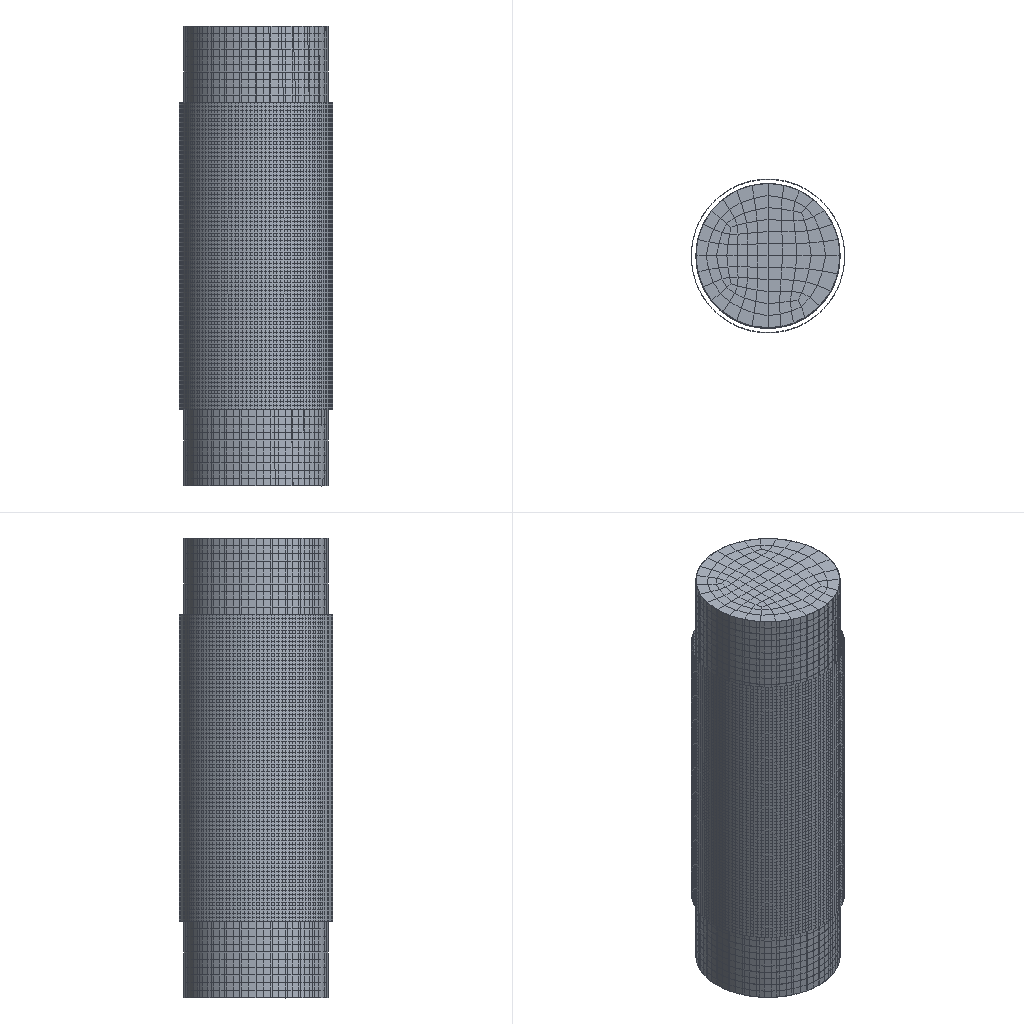Simulation study | abaqus
Set-up summary:
category,name,step,type,value,unit,region
solver,abaqus
solver,version,,,Abaqus/Standard 2020
units,not stated in the deck,,not stated
analysis,deck,,static,static
load_step,Step-1,Step-1,static,nlgeom=True
contact,interactions,,,general=1 pairs=0 ties=1
load_step,requested,,,1
mesh,nodes,,,19323
mesh,elements,,,18438
element_type,S4,,shell,14280
element_type,C3D8,,solid,3540
element_type,R3D3,,rigid,8
element_type,R3D4,,rigid,610
load,load commands in deck,,count,1
bc,support commands in deck,,count,7
material,CONCRETE,,in results
material,PLATE,,in results
material,STEEL,,in results
material,T300/M18,,in results
check,setup vs results,,match,"per instance, exact: element labels, types and connectivity; labels of the nodes the elements use; coordinates of those nodes at SINGLE_PRECISION in 2 of 5 instance(s)"
Abaqus input file, long lists of numbers shortened:
*Heading
** Job name: Job-2 Model name: 3-F1-D-Copy
** Generated by: Abaqus/CAE 2020
*Preprint, echo=NO, model=NO, history=NO, contact=NO
**
** PARTS
**
*Part, name=CFRP
*Node
      1,          50.,           0.,          75.
      2,          50.,           0.,         125.
** (10204 more lines like these left out)
*Element, type=S4
    1,     1,     5,   505,   630
    2,     5,     6,   506,   505
** (10078 more lines like these left out)
*Elset, elset=COMPOSITELAYUP-1-1, generate
     1,  10080,      1
** Region: (COMPOSITELAYUP-1-1: Generated From Layup)
*Elset, elset=COMPOSITELAYUP-1-1-1, generate
     1,  10080,      1
** Section: COMPOSITELAYUP-1-1
*Shell Section, elset=COMPOSITELAYUP-1-1-1, composite, offset=SNEG, layup=COMPOSITELAYUP-1
0.3, 5, T300/M18, 0., 层-1
*End Part
**
*Part, name=con
*Node
      1,           0.,           0.,         300.
      2,           0.,         -47.,         300.
** (4121 more lines like these left out)
*Element, type=C3D8
  1,  407,  408, 1902, 1729,   14,   15,  245,  244
  2,  408,  409, 1903, 1902,   15,   16,  246,  245
** (3538 more lines like these left out)
*Nset, nset=Set-8, generate
    1,  4123,     1
*Elset, elset=Set-8, generate
    1,  3540,     1
** Section: Section-1-_PICKEDSET2
*Solid Section, elset=Set-8, material=CONCRETE
,
*End Part
**
*Part, name="perforated steel"
*Node
      1,  -40.703,        -23.5,         125.
      2,  -30.256,  -35.967,    141.256
** (4372 more lines like these left out)
*Element, type=S4
   1,    1,   63,  919,   82
   2,   63,   64,  920,  919
** (4198 more lines like these left out)
*Nset, nset=_PICKEDSET2_#2, internal, generate
    1,  4374,     1
*Elset, elset=_PICKEDSET2_#2, internal, generate
    1,  4200,     1
*Nset, nset="Edge Seeds-3"
   2,   3,   4,   7,  10,  11,  13,  15,  17,  18,  20,  22,  24,  25,  27,  28
  30,  32,  33,  35,  36,  38,  40,  41,  43,  44,  45,  46,  47,  48,  67,  68
** (13 more lines like these left out)
*Elset, elset="Edge Seeds-3"
    5,   10,   15,   20,   25,   30,   35,   40,   45,   50,   51,   56,   61,   66,   71,   76
   81,   86,   91,   96,  101,  106,  111,  116,  121,  126,  131,  136,  141,  146,  151,  156
** (13 more lines like these left out)
** Section: Section-2-_PICKEDSET2_#2
*Shell Section, elset=_PICKEDSET2_#2, material=STEEL, offset=SNEG
3., 9
*End Part
**
*Part, name=rigid
*Node
      1,   48.014,  -57.617,          40.
      2,   48.014,  -57.617,           0.
** (307 more lines like these left out)
*Element, type=R3D4
 1,   1,   3,  63,  93
 2,   3,   4,  64,  63
** (303 more lines like these left out)
*Element, type=R3D3
94, 182, 212, 165
95, 192, 191, 181
** (2 more lines like these left out)
*Node
    310,           0., -4.59242545e-15,          40.
*Nset, nset=rigid-RefPt_, internal
310,
*Elset, elset=rigid, generate
   1,  309,    1
*End Part
**
**
** ASSEMBLY
**
*Assembly, name=Assembly
**
*Instance, name="perforated steel-1", part="perforated steel"
*End Instance
**
*Instance, name=CFRP-1, part=CFRP
          0.,           0.,          50.
*End Instance
**
*Instance, name=con-1, part=con
*End Instance
**
*Instance, name=rigid-1, part=rigid
          0.,           0.,         -40.
*End Instance
**
*Instance, name=rigid-2, part=rigid
          0.,           0.,         300.
*End Instance
**
*Nset, nset=Set-35, instance=rigid-2
 310,
*Nset, nset=Set-36, instance=rigid-1
 310,
*Elset, elset=__PICKEDSURF62_E3, internal, instance="perforated steel-1"
 2291, 2292, 2293, 2294, 2295, 2296, 2297, 2298, 2299, 2300, 2791, 2792, 2793, 2794, 2795, 2796
 2797, 2798, 2799, 2800, 3291, 3292, 3293, 3294, 3295, 3296, 3297, 3298, 3299, 3300, 3591, 3592
** (2 more lines like these left out)
*Elset, elset=__PICKEDSURF63_E3, internal, instance="perforated steel-1"
 1141, 1142, 1143, 1144, 1145, 1146, 1147, 1148, 1149, 1150, 1441, 1442, 1443, 1444, 1445, 1446
 1447, 1448, 1449, 1450, 1741, 1742, 1743, 1744, 1745, 1746, 1747, 1748, 1749, 1750, 2041, 2042
** (2 more lines like these left out)
*Elset, elset=__PICKEDSURF64_SNEG, internal, instance="perforated steel-1", generate
    1,  4200,     1
*Elset, elset=__PICKEDSURF71_SPOS, internal, instance="perforated steel-1"
    1,    2,    3,    4,    5,    6,    7,    8,    9,   10,   11,   12,   13,   14,   15,   16
   17,   18,   19,   20,   21,   22,   23,   24,   25,   26,   27,   28,   29,   30,   31,   32
** (73 more lines like these left out)
*Elset, elset=__PICKEDSURF72_SPOS, internal, instance="perforated steel-1"
  901,  902,  903,  904,  905,  906,  907,  908,  909,  910,  911,  912,  913,  914,  915,  916
  917,  918,  919,  920,  921,  922,  923,  924,  925,  926,  927,  928,  929,  930,  931,  932
** (92 more lines like these left out)
*Elset, elset=__PICKEDSURF73_SNEG, internal, instance=CFRP-1, generate
  6301,  10080,      1
*Elset, elset=__PICKEDSURF74_SNEG, internal, instance=CFRP-1, generate
    1,  2520,     1
*Elset, elset=__PICKEDSURF75_SPOS, internal, instance="perforated steel-1"
 2051, 2052, 2053, 2054, 2055, 2056, 2057, 2058, 2059, 2060, 2061, 2062, 2063, 2064, 2065, 2066
 2067, 2068, 2069, 2070, 2071, 2072, 2073, 2074, 2075, 2076, 2077, 2078, 2079, 2080, 2081, 2082
** (92 more lines like these left out)
*Elset, elset=__PICKEDSURF76_SNEG, internal, instance=CFRP-1, generate
 2521,  6300,     1
*Elset, elset=_m_Surf-6_E3, internal, instance="perforated steel-1"
 1141, 1142, 1143, 1144, 1145, 1146, 1147, 1148, 1149, 1150, 1441, 1442, 1443, 1444, 1445, 1446
 1447, 1448, 1449, 1450, 1741, 1742, 1743, 1744, 1745, 1746, 1747, 1748, 1749, 1750, 2041, 2042
** (6 more lines like these left out)
*Surface, type=ELEMENT, name=m_Surf-6
_m_Surf-6_E3, E3
*Elset, elset=_m_Surf-8_SPOS, internal, instance="perforated steel-1", generate
    1,  4200,     1
*Surface, type=ELEMENT, name=m_Surf-8
_m_Surf-8_SPOS, SPOS
*Elset, elset=_s_Surf-7_SNEG, internal, instance="perforated steel-1", generate
    1,  4200,     1
*Surface, type=ELEMENT, name=s_Surf-7
_s_Surf-7_SNEG, SNEG
*Elset, elset=_s_Surf-8_SNEG, internal, instance=CFRP-1, generate
     1,  10080,      1
*Surface, type=ELEMENT, name=s_Surf-8
_s_Surf-8_SNEG, SNEG
*Rigid Body, ref node=rigid-1.rigid-RefPt_, elset=rigid-1.rigid
*Rigid Body, ref node=rigid-2.rigid-RefPt_, elset=rigid-2.rigid
** Constraint: Constraint-3
*Tie, name=Constraint-3, adjust=yes
s_Surf-8, m_Surf-8
*Elset, elset=__Int-1_gcs0_11_S3, internal, instance=con-1
  781,  782,  783,  790,  791,  792,  799,  800,  801,  808,  809,  810,  817,  818,  819,  826
  827,  828,  835,  836,  837,  844,  845,  846,  853,  854,  855,  862,  863,  864,  871,  872
** (4 more lines like these left out)
*Elset, elset=__Int-1_gcs0_11_S4, internal, instance=con-1
 1098, 1101, 1104, 1107, 1110, 1113, 1116, 1119, 1122, 1125, 1128, 1131, 1134, 1137, 1140, 1143
 1146, 1149, 1152, 1155, 1158, 1161, 1164, 1167, 1170, 1173, 1176, 1179, 1182, 1185, 1188, 1191
** (6 more lines like these left out)
*Surface, type=ELEMENT, name=_Int-1_gcs0_11, internal
__Int-1_gcs0_11_S3, S3
__Int-1_gcs0_11_S4, S4
*Elset, elset=__Int-1_gcs0_12_S4, internal, instance=con-1
 182, 184, 186, 188, 190, 192, 194, 196, 198, 200, 202, 204, 206, 208, 210, 212
 214, 216, 218, 220, 222, 224, 226, 228, 230, 232, 234, 236, 238, 240, 242, 244
** (8 more lines like these left out)
*Elset, elset=__Int-1_gcs0_12_S3, internal, instance=con-1
 271, 272, 273, 274, 279, 280, 281, 282, 287, 288, 289, 290, 295, 296, 297, 298
 303, 304, 305, 306, 311, 312, 313, 314, 319, 320, 321, 322, 327, 328, 329, 330
** (2 more lines like these left out)
*Surface, type=ELEMENT, name=_Int-1_gcs0_12, internal
__Int-1_gcs0_12_S4, S4
__Int-1_gcs0_12_S3, S3
*Elset, elset=__Int-1_gcs0_13_S4, internal, instance=con-1
 2733, 2736, 2739, 2742, 2745, 2748, 2751, 2754, 2757, 2760, 2763, 2766, 2769, 2772, 2775, 2778
 2781, 2784, 2787, 2790, 2793, 2796, 2799, 2802, 2805, 2808, 2811, 2814, 2817, 2820, 2823, 2826
** (6 more lines like these left out)
*Elset, elset=__Int-1_gcs0_13_S3, internal, instance=con-1
 2911, 2912, 2913, 2920, 2921, 2922, 2929, 2930, 2931, 2938, 2939, 2940, 2947, 2948, 2949, 2956
 2957, 2958, 2965, 2966, 2967, 2974, 2975, 2976, 2983, 2984, 2985, 2992, 2993, 2994, 3001, 3002
** (4 more lines like these left out)
*Surface, type=ELEMENT, name=_Int-1_gcs0_13, internal
__Int-1_gcs0_13_S4, S4
__Int-1_gcs0_13_S3, S3
*Elset, elset=__Int-1_gcs0_14_S3, internal, instance=con-1
 1771, 1772, 1773, 1777, 1778, 1779, 1783, 1784, 1785, 1789, 1790, 1791, 1795, 1796, 1797, 1801
 1802, 1803, 1807, 1808, 1809, 1813, 1814, 1815, 1819, 1820, 1821, 1825, 1826, 1827, 1831, 1832
** (4 more lines like these left out)
*Elset, elset=__Int-1_gcs0_14_S4, internal, instance=con-1
 2042, 2044, 2046, 2048, 2050, 2052, 2054, 2056, 2058, 2060, 2062, 2064, 2066, 2068, 2070, 2072
 2074, 2076, 2078, 2080, 2082, 2084, 2086, 2088, 2090, 2092, 2094, 2096, 2098, 2100, 2102, 2104
** (6 more lines like these left out)
*Surface, type=ELEMENT, name=_Int-1_gcs0_14, internal
__Int-1_gcs0_14_S3, S3
__Int-1_gcs0_14_S4, S4
*Elset, elset=__Int-1_gcs0_17_SPOS, internal, instance=rigid-1, generate
  1,  93,   1
*Surface, type=ELEMENT, name=_Int-1_gcs0_17, internal
__Int-1_gcs0_17_SPOS, SPOS
*Elset, elset=__Int-1_gcs0_20_SNEG, internal, instance=rigid-1, generate
  1,  93,   1
*Surface, type=ELEMENT, name=_Int-1_gcs0_20, internal
__Int-1_gcs0_20_SNEG, SNEG
*Elset, elset=__Int-1_gcs0_23_SPOS, internal, instance=rigid-2, generate
  1,  93,   1
*Surface, type=ELEMENT, name=_Int-1_gcs0_23, internal
__Int-1_gcs0_23_SPOS, SPOS
*Elset, elset=__Int-1_gcs0_26_SNEG, internal, instance=rigid-2, generate
  1,  93,   1
*Surface, type=ELEMENT, name=_Int-1_gcs0_26, internal
__Int-1_gcs0_26_SNEG, SNEG
*End Assembly
*Amplitude, name=Amp-1
             0.,              0.,              1.,              1.
**
** MATERIALS
**
**   It was tested in lab that average compressive strength is 46.2 MPa
*Material, name=CONCRETE
*Density
 2.27e-09,
*Elastic
 28394.4, 0.2
*Concrete Damaged Plasticity
30.,     0.1,    1.16, 0.6667,   1e-06
*Concrete Compression Hardening
  10.216,     0.
  14.851, 0.0002
 19.037, 0.0004
 22.773, 0.0006
 26.06, 0.0008
 28.898,  0.001
 31.287, 0.0012
 33.226, 0.0014
 34.716, 0.0016
 35.757, 0.0018
 36.348,  0.002
 36.496, 0.0022
 36.44, 0.0024
 36.315, 0.0026
 36.135, 0.0028
 35.911,  0.003
 35.654, 0.0032
 35.369, 0.0034
 35.064, 0.0036
 34.742, 0.0038
 34.407,  0.004
  34.064, 0.0042
 33.714, 0.0044
 33.36, 0.0046
 33.003, 0.0048
 32.645,  0.005
 31.753, 0.0055
 30.876,  0.006
 30.021, 0.0065
 29.194,  0.007
 28.397, 0.0075
 27.631,  0.008
 26.897, 0.0085
 26.194,  0.009
 25.521, 0.0095
 24.878,   0.01
 24.262, 0.0105
 23.673,  0.011
 23.11, 0.0115
 22.57,  0.012
** (176 more lines like these left out)
*Concrete Tension Stiffening
 3.32,      0.
 1.92,   2e-05
 1.72,   4e-05
 1.53,   6e-05
 1.37,   8e-05
 1.24,  0.0001
 1.13, 0.00011
 1.04, 0.00013
 0.97, 0.00015
  0.9, 0.00016
 0.85, 0.00018
*Material, name=PLATE
*Elastic
 1e+15, 1e-08
**   Stainless Steel - Grade 310
*Material, name=STEEL
*Density
 7.84e-09,
*Elastic
206000., 0.3
*Plastic
    176.,       0.
 185.697,    5e-05
 194.189,   0.0001
 201.475,  0.00015
 207.555,   0.0002
  212.43,  0.00025
   216.1,   0.0003
 218.564,  0.00035
 219.822,   0.0004
    220., 0.000627
    220., 0.001127
    220., 0.001627
    220., 0.002127
    220., 0.002627
    220., 0.003127
    220., 0.003627
    220., 0.004127
    220., 0.004627
    220., 0.005127
    220., 0.005627
    220., 0.006127
    220., 0.006627
    220., 0.007127
    220., 0.007627
    220., 0.008127
    220., 0.008627
    220., 0.009127
    220., 0.009627
    220., 0.01013
    220., 0.01063
    220., 0.01113
    220., 0.01163
 220.343, 0.01226
 226.066, 0.01726
 231.788, 0.02226
  237.51, 0.02726
 243.232, 0.03226
 248.954, 0.03726
 254.677, 0.04226
 260.399, 0.04726
** (26 more lines like these left out)
*Material, name=T300/M18
*Damage Initiation, criterion=HASHIN
2050.,1200.,  62., 190.,  81.,  81.
*Density
 1.76e-09,
*Elastic, type=LAMINA
170000.,9000., 0.34,4800.,4800.,4500.
**
** INTERACTION PROPERTIES
**
*Surface Interaction, name=INTPROP-1
1.,
*Friction, slip tolerance=0.005
 0.25,
*Surface Behavior, pressure-overclosure=HARD
**
** INTERACTIONS
**
** Interaction: Int-1
*Contact
*Contact Inclusions, ALL EXTERIOR
*Contact Property Assignment
 ,  , INTPROP-1
*Surface Property Assignment, property=GEOMETRIC CORRECTION
_Int-1_gcs0_11, Circumferential, 0., 0., 0.,  0., 0., 1.
_Int-1_gcs0_12, Circumferential, 0., 0., 0.,  0., 0., 1.
_Int-1_gcs0_13, Circumferential, 0., 0., 0.,  0., 0., 1.
_Int-1_gcs0_14, Circumferential, 0., 0., 0.,  0., 0., 1.
_Int-1_gcs0_17, Circumferential, 0., 0., -40.,  0., 0., -39.
_Int-1_gcs0_20, Circumferential, 0., 0., -40.,  0., 0., -39.
_Int-1_gcs0_23, Circumferential, 0., 0., 300.,  0., 0., 301.
_Int-1_gcs0_26, Circumferential, 0., 0., 300.,  0., 0., 301.
** ----------------------------------------------------------------
**
** STEP: Step-1
**
*Step, name=Step-1, nlgeom=YES, inc=1000
*Static, stabilize=0.0002, allsdtol=0.05, continue=NO
0.01, 1., 1e-05, 1.
**
** BOUNDARY CONDITIONS
**
** Name: BC-1 Type: 对称/反对称/完全固定
*Boundary
Set-35, ENCASTRE
** Name: BC-2 Type: 位移/转角
*Boundary, amplitude=Amp-1
Set-36, 1, 1
Set-36, 2, 2
Set-36, 3, 3, 10.
Set-36, 4, 4
Set-36, 5, 5
Set-36, 6, 6
**
** OUTPUT REQUESTS
**
*Restart, write, frequency=0
**
** FIELD OUTPUT: F-Output-3
**
*Output, field
*Element Output, directions=YES
STATUS,
*Contact Output
CDISP, CSTRESS
**
** FIELD OUTPUT: F-Output-1
**
*Node Output
CF, RF, U
**
** FIELD OUTPUT: F-Output-2
**
*Element Output, directions=YES
DAMAGEC, DAMAGET, DMICRT, HSNFCCRT, HSNFTCRT, HSNMCCRT, HSNMTCRT, LE, PE, PEEQ, PEMAG, S, SDEG, STATUS
**
** HISTORY OUTPUT: H-Output-1
**
*Output, history
*Node Output, nset=Set-36
RF3,
**
** HISTORY OUTPUT: H-Output-2
**
*Node Output, nset=Set-36
U3,
*End Step
Results summary:
result,step,,completed,increments=11 time=1.0/1.0
result,analysis,,,static
result,last_loadstep,,,1
result,analysis steps,,count,1
result,primary field,,,"U, UR"
result,reaction total,,FX,-19.659,model units
result,reaction total,,FY,1.54,model units
result,reaction total,,FZ,10875.062,model units